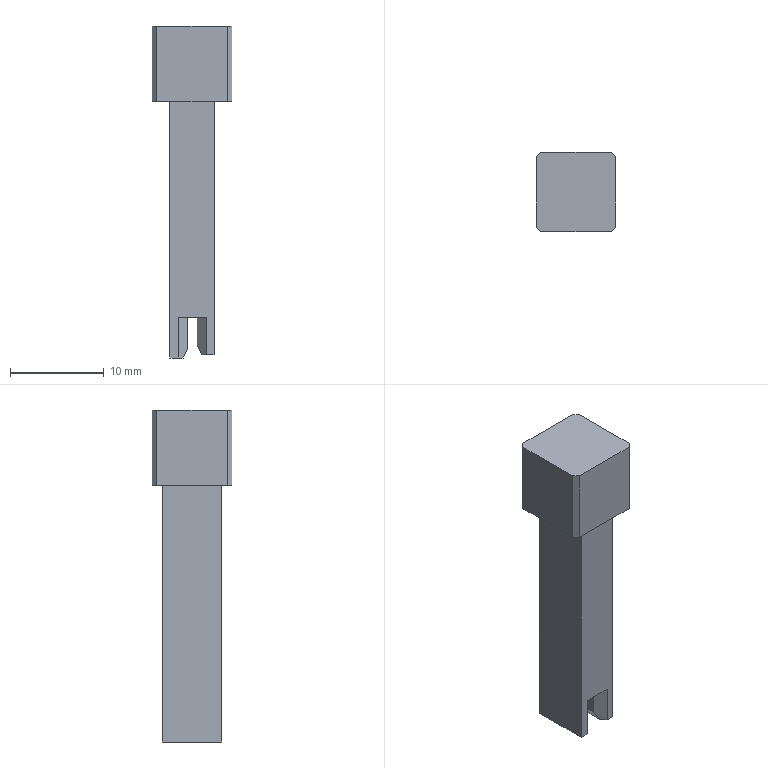Part | STEP file | Riveting press block | 1 solid | 25 faces | box 8.5 x 8.5 x 35.35 mm | volume 1342 mm3 | plane 25